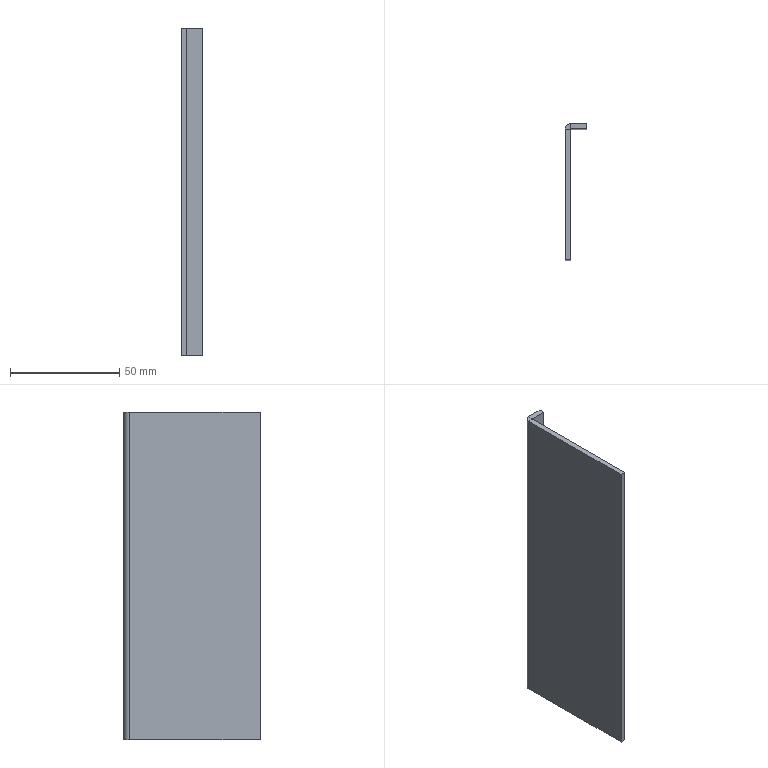Part | SolidWorks | features FlatPattern 1, SMBaseFlange 1, SheetMetal 1 | 1 solid | 14 faces | box 10 x 62.5 x 150 mm | volume 26033 mm3 | plane 12 | cylinder 2 | commonest cylinder face diameters 0.2 x1 5.2 x1
STEP:
#1=CARTESIAN_POINT('',(-7.4,0.,150.));
#2=VERTEX_POINT('',#1);
#3=CARTESIAN_POINT('',(-7.4,-2.5,150.));
#4=VERTEX_POINT('',#3);
#5=CARTESIAN_POINT('',(-7.4,0.,150.));
#6=DIRECTION('',(0.,-1.,0.));
#7=VECTOR('',#6,1000.);
#8=LINE('',#5,#7);
#9=EDGE_CURVE('',#2,#4,#8,.T.);
#10=ORIENTED_EDGE('',*,*,#9,.F.);
#11=CARTESIAN_POINT('',(-10.,-2.6,150.));
#12=VERTEX_POINT('',#11);
#13=CARTESIAN_POINT('',(-7.4,-2.6,150.));
#14=DIRECTION('',(0.,0.,1.));
#15=DIRECTION('',(-1.,0.,0.));
#16=AXIS2_PLACEMENT_3D('',#13,#14,#15);
#17=CIRCLE('',#16,2.6);
#18=EDGE_CURVE('',#2,#12,#17,.T.);
#19=ORIENTED_EDGE('',*,*,#18,.T.);
#20=CARTESIAN_POINT('',(-7.5,-2.6,150.));
#21=VERTEX_POINT('',#20);
#22=CARTESIAN_POINT('',(-7.5,-2.6,150.));
#23=DIRECTION('',(-1.,0.,0.));
#24=VECTOR('',#23,1000.);
#25=LINE('',#22,#24);
#26=EDGE_CURVE('',#21,#12,#25,.T.);
#27=ORIENTED_EDGE('',*,*,#26,.F.);
#28=CARTESIAN_POINT('',(-7.4,-2.6,150.));
#29=DIRECTION('',(0.,0.,1.));
#30=DIRECTION('',(1.,0.,0.));
#31=AXIS2_PLACEMENT_3D('',#28,#29,#30);
#32=CIRCLE('',#31,0.1);
#33=EDGE_CURVE('',#4,#21,#32,.T.);
#34=ORIENTED_EDGE('',*,*,#33,.F.);
#35=EDGE_LOOP('',(#10,#19,#27,#34));
#36=FACE_OUTER_BOUND('',#35,.T.);
#37=CARTESIAN_POINT('',(-7.4,0.,150.));
#38=DIRECTION('',(0.,0.,1.));
#39=DIRECTION('',(1.,0.,0.));
#40=AXIS2_PLACEMENT_3D('',#37,#38,#39);
#41=PLANE('',#40);
#42=ADVANCED_FACE('',(#36),#41,.T.);
#43=CARTESIAN_POINT('',(0.,0.,150.));
#44=VERTEX_POINT('',#43);
#45=CARTESIAN_POINT('',(0.,0.,150.));
#46=DIRECTION('',(-1.,0.,0.));
#47=VECTOR('',#46,1000.);
#48=LINE('',#45,#47);
#49=EDGE_CURVE('',#44,#2,#48,.T.);
#50=ORIENTED_EDGE('',*,*,#49,.T.);
#51=ORIENTED_EDGE('',*,*,#9,.T.);
#52=CARTESIAN_POINT('',(0.,-2.5,150.));
#53=VERTEX_POINT('',#52);
#54=CARTESIAN_POINT('',(0.,-2.5,150.));
#55=DIRECTION('',(-1.,0.,0.));
#56=VECTOR('',#55,1000.);
#57=LINE('',#54,#56);
#58=EDGE_CURVE('',#53,#4,#57,.T.);
#59=ORIENTED_EDGE('',*,*,#58,.F.);
#60=CARTESIAN_POINT('',(0.,0.,150.));
#61=DIRECTION('',(0.,-1.,0.));
#62=VECTOR('',#61,1000.);
#63=LINE('',#60,#62);
#64=EDGE_CURVE('',#44,#53,#63,.T.);
#65=ORIENTED_EDGE('',*,*,#64,.F.);
#66=EDGE_LOOP('',(#50,#51,#59,#65));
#67=FACE_OUTER_BOUND('',#66,.T.);
#68=CARTESIAN_POINT('',(-7.5,-2.6,150.));
#69=DIRECTION('',(0.,0.,1.));
#70=DIRECTION('',(1.,0.,0.));
#71=AXIS2_PLACEMENT_3D('',#68,#69,#70);
#72=PLANE('',#71);
#73=ADVANCED_FACE('',(#67),#72,.T.);
#74=CARTESIAN_POINT('',(-10.,-2.6,0.));
#75=VERTEX_POINT('',#74);
#76=CARTESIAN_POINT('',(-7.5,-2.6,0.));
#77=VERTEX_POINT('',#76);
#78=CARTESIAN_POINT('',(-10.,-2.6,0.));
#79=DIRECTION('',(1.,0.,0.));
#80=VECTOR('',#79,1000.);
#81=LINE('',#78,#80);
#82=EDGE_CURVE('',#75,#77,#81,.T.);
#83=ORIENTED_EDGE('',*,*,#82,.F.);
#84=CARTESIAN_POINT('',(-7.4,0.,0.));
#85=VERTEX_POINT('',#84);
#86=CARTESIAN_POINT('',(-7.4,-2.6,0.));
#87=DIRECTION('',(0.,0.,1.));
#88=DIRECTION('',(-1.,0.,0.));
#89=AXIS2_PLACEMENT_3D('',#86,#87,#88);
#90=CIRCLE('',#89,2.6);
#91=EDGE_CURVE('',#85,#75,#90,.T.);
#92=ORIENTED_EDGE('',*,*,#91,.F.);
#93=CARTESIAN_POINT('',(-7.4,-2.5,0.));
#94=VERTEX_POINT('',#93);
#95=CARTESIAN_POINT('',(-7.4,-2.5,0.));
#96=DIRECTION('',(0.,1.,0.));
#97=VECTOR('',#96,1000.);
#98=LINE('',#95,#97);
#99=EDGE_CURVE('',#94,#85,#98,.T.);
#100=ORIENTED_EDGE('',*,*,#99,.F.);
#101=CARTESIAN_POINT('',(-7.4,-2.6,0.));
#102=DIRECTION('',(0.,0.,1.));
#103=DIRECTION('',(1.,0.,0.));
#104=AXIS2_PLACEMENT_3D('',#101,#102,#103);
#105=CIRCLE('',#104,0.1);
#106=EDGE_CURVE('',#94,#77,#105,.T.);
#107=ORIENTED_EDGE('',*,*,#106,.T.);
#108=EDGE_LOOP('',(#83,#92,#100,#107));
#109=FACE_OUTER_BOUND('',#108,.T.);
#110=CARTESIAN_POINT('',(-10.,-2.6,0.));
#111=DIRECTION('',(0.,0.,-1.));
#112=DIRECTION('',(-1.,0.,0.));
#113=AXIS2_PLACEMENT_3D('',#110,#111,#112);
#114=PLANE('',#113);
#115=ADVANCED_FACE('',(#109),#114,.T.);
#116=CARTESIAN_POINT('',(-10.,-62.5,0.));
#117=VERTEX_POINT('',#116);
#118=CARTESIAN_POINT('',(-10.,0.,0.));
#119=DIRECTION('',(0.,-1.,0.));
#120=VECTOR('',#119,1000.);
#121=LINE('',#118,#120);
#122=EDGE_CURVE('',#75,#117,#121,.T.);
#123=ORIENTED_EDGE('',*,*,#122,.F.);
#124=ORIENTED_EDGE('',*,*,#82,.T.);
#125=CARTESIAN_POINT('',(-7.5,-62.5,0.));
#126=VERTEX_POINT('',#125);
#127=CARTESIAN_POINT('',(-7.5,0.,0.));
#128=DIRECTION('',(0.,-1.,0.));
#129=VECTOR('',#128,1000.);
#130=LINE('',#127,#129);
#131=EDGE_CURVE('',#77,#126,#130,.T.);
#132=ORIENTED_EDGE('',*,*,#131,.T.);
#133=CARTESIAN_POINT('',(-7.5,-62.5,0.));
#134=DIRECTION('',(-1.,0.,0.));
#135=VECTOR('',#134,1000.);
#136=LINE('',#133,#135);
#137=EDGE_CURVE('',#126,#117,#136,.T.);
#138=ORIENTED_EDGE('',*,*,#137,.T.);
#139=EDGE_LOOP('',(#123,#124,#132,#138));
#140=FACE_OUTER_BOUND('',#139,.T.);
#141=CARTESIAN_POINT('',(-7.4,-2.5,0.));
#142=DIRECTION('',(0.,0.,-1.));
#143=DIRECTION('',(-1.,0.,0.));
#144=AXIS2_PLACEMENT_3D('',#141,#142,#143);
#145=PLANE('',#144);
#146=ADVANCED_FACE('',(#140),#145,.T.);
#147=ORIENTED_EDGE('',*,*,#122,.T.);
#148=CARTESIAN_POINT('',(-10.,-62.5,150.));
#149=VERTEX_POINT('',#148);
#150=CARTESIAN_POINT('',(-10.,-62.5,150.));
#151=DIRECTION('',(0.,0.,-1.));
#152=VECTOR('',#151,1000.);
#153=LINE('',#150,#152);
#154=EDGE_CURVE('',#149,#117,#153,.T.);
#155=ORIENTED_EDGE('',*,*,#154,.F.);
#156=CARTESIAN_POINT('',(-10.,0.,150.));
#157=DIRECTION('',(0.,-1.,0.));
#158=VECTOR('',#157,1000.);
#159=LINE('',#156,#158);
#160=EDGE_CURVE('',#12,#149,#159,.T.);
#161=ORIENTED_EDGE('',*,*,#160,.F.);
#162=CARTESIAN_POINT('',(-10.,-2.6,150.));
#163=DIRECTION('',(0.,0.,-1.));
#164=VECTOR('',#163,1000.);
#165=LINE('',#162,#164);
#166=EDGE_CURVE('',#12,#75,#165,.T.);
#167=ORIENTED_EDGE('',*,*,#166,.T.);
#168=EDGE_LOOP('',(#147,#155,#161,#167));
#169=FACE_OUTER_BOUND('',#168,.T.);
#170=CARTESIAN_POINT('',(-10.,0.,150.));
#171=DIRECTION('',(1.,0.,0.));
#172=DIRECTION('',(0.,1.,0.));
#173=AXIS2_PLACEMENT_3D('',#170,#171,#172);
#174=PLANE('',#173);
#175=ADVANCED_FACE('',(#169),#174,.F.);
#176=ORIENTED_EDGE('',*,*,#137,.F.);
#177=CARTESIAN_POINT('',(-7.5,-62.5,150.));
#178=VERTEX_POINT('',#177);
#179=CARTESIAN_POINT('',(-7.5,-62.5,150.));
#180=DIRECTION('',(0.,0.,-1.));
#181=VECTOR('',#180,1000.);
#182=LINE('',#179,#181);
#183=EDGE_CURVE('',#178,#126,#182,.T.);
#184=ORIENTED_EDGE('',*,*,#183,.F.);
#185=CARTESIAN_POINT('',(-7.5,-62.5,150.));
#186=DIRECTION('',(-1.,0.,0.));
#187=VECTOR('',#186,1000.);
#188=LINE('',#185,#187);
#189=EDGE_CURVE('',#178,#149,#188,.T.);
#190=ORIENTED_EDGE('',*,*,#189,.T.);
#191=ORIENTED_EDGE('',*,*,#154,.T.);
#192=EDGE_LOOP('',(#176,#184,#190,#191));
#193=FACE_OUTER_BOUND('',#192,.T.);
#194=CARTESIAN_POINT('',(-7.5,-62.5,150.));
#195=DIRECTION('',(0.,-1.,0.));
#196=DIRECTION('',(0.,0.,-1.));
#197=AXIS2_PLACEMENT_3D('',#194,#195,#196);
#198=PLANE('',#197);
#199=ADVANCED_FACE('',(#193),#198,.T.);
#200=ORIENTED_EDGE('',*,*,#131,.F.);
#201=CARTESIAN_POINT('',(-7.5,-2.6,150.));
#202=DIRECTION('',(0.,0.,-1.));
#203=VECTOR('',#202,1000.);
#204=LINE('',#201,#203);
#205=EDGE_CURVE('',#21,#77,#204,.T.);
#206=ORIENTED_EDGE('',*,*,#205,.F.);
#207=CARTESIAN_POINT('',(-7.5,0.,150.));
#208=DIRECTION('',(0.,-1.,0.));
#209=VECTOR('',#208,1000.);
#210=LINE('',#207,#209);
#211=EDGE_CURVE('',#21,#178,#210,.T.);
#212=ORIENTED_EDGE('',*,*,#211,.T.);
#213=ORIENTED_EDGE('',*,*,#183,.T.);
#214=EDGE_LOOP('',(#200,#206,#212,#213));
#215=FACE_OUTER_BOUND('',#214,.T.);
#216=CARTESIAN_POINT('',(-7.5,0.,150.));
#217=DIRECTION('',(1.,0.,0.));
#218=DIRECTION('',(0.,1.,0.));
#219=AXIS2_PLACEMENT_3D('',#216,#217,#218);
#220=PLANE('',#219);
#221=ADVANCED_FACE('',(#215),#220,.T.);
#222=ORIENTED_EDGE('',*,*,#106,.F.);
#223=CARTESIAN_POINT('',(-7.4,-2.5,150.));
#224=DIRECTION('',(0.,0.,-1.));
#225=VECTOR('',#224,1000.);
#226=LINE('',#223,#225);
#227=EDGE_CURVE('',#4,#94,#226,.T.);
#228=ORIENTED_EDGE('',*,*,#227,.F.);
#229=ORIENTED_EDGE('',*,*,#33,.T.);
#230=ORIENTED_EDGE('',*,*,#205,.T.);
#231=EDGE_LOOP('',(#222,#228,#229,#230));
#232=FACE_OUTER_BOUND('',#231,.T.);
#233=CARTESIAN_POINT('',(-7.4,-2.6,150.));
#234=DIRECTION('',(0.,0.,-1.));
#235=DIRECTION('',(-1.,0.,0.));
#236=AXIS2_PLACEMENT_3D('',#233,#234,#235);
#237=CYLINDRICAL_SURFACE('',#236,0.1);
#238=ADVANCED_FACE('',(#232),#237,.F.);
#239=CARTESIAN_POINT('',(0.,-2.5,0.));
#240=VERTEX_POINT('',#239);
#241=CARTESIAN_POINT('',(0.,-2.5,0.));
#242=DIRECTION('',(-1.,0.,0.));
#243=VECTOR('',#242,1000.);
#244=LINE('',#241,#243);
#245=EDGE_CURVE('',#240,#94,#244,.T.);
#246=ORIENTED_EDGE('',*,*,#245,.F.);
#247=CARTESIAN_POINT('',(0.,-2.5,150.));
#248=DIRECTION('',(0.,0.,-1.));
#249=VECTOR('',#248,1000.);
#250=LINE('',#247,#249);
#251=EDGE_CURVE('',#53,#240,#250,.T.);
#252=ORIENTED_EDGE('',*,*,#251,.F.);
#253=ORIENTED_EDGE('',*,*,#58,.T.);
#254=ORIENTED_EDGE('',*,*,#227,.T.);
#255=EDGE_LOOP('',(#246,#252,#253,#254));
#256=FACE_OUTER_BOUND('',#255,.T.);
#257=CARTESIAN_POINT('',(0.,-2.5,150.));
#258=DIRECTION('',(0.,-1.,0.));
#259=DIRECTION('',(1.,0.,0.));
#260=AXIS2_PLACEMENT_3D('',#257,#258,#259);
#261=PLANE('',#260);
#262=ADVANCED_FACE('',(#256),#261,.T.);
#263=CARTESIAN_POINT('',(0.,0.,0.));
#264=VERTEX_POINT('',#263);
#265=CARTESIAN_POINT('',(0.,0.,0.));
#266=DIRECTION('',(0.,-1.,0.));
#267=VECTOR('',#266,1000.);
#268=LINE('',#265,#267);
#269=EDGE_CURVE('',#264,#240,#268,.T.);
#270=ORIENTED_EDGE('',*,*,#269,.F.);
#271=CARTESIAN_POINT('',(0.,0.,150.));
#272=DIRECTION('',(0.,0.,-1.));
#273=VECTOR('',#272,1000.);
#274=LINE('',#271,#273);
#275=EDGE_CURVE('',#44,#264,#274,.T.);
#276=ORIENTED_EDGE('',*,*,#275,.F.);
#277=ORIENTED_EDGE('',*,*,#64,.T.);
#278=ORIENTED_EDGE('',*,*,#251,.T.);
#279=EDGE_LOOP('',(#270,#276,#277,#278));
#280=FACE_OUTER_BOUND('',#279,.T.);
#281=CARTESIAN_POINT('',(0.,0.,150.));
#282=DIRECTION('',(1.,0.,0.));
#283=DIRECTION('',(0.,1.,0.));
#284=AXIS2_PLACEMENT_3D('',#281,#282,#283);
#285=PLANE('',#284);
#286=ADVANCED_FACE('',(#280),#285,.T.);
#287=CARTESIAN_POINT('',(0.,0.,0.));
#288=DIRECTION('',(-1.,0.,0.));
#289=VECTOR('',#288,1000.);
#290=LINE('',#287,#289);
#291=EDGE_CURVE('',#264,#85,#290,.T.);
#292=ORIENTED_EDGE('',*,*,#291,.T.);
#293=CARTESIAN_POINT('',(-7.4,0.,150.));
#294=DIRECTION('',(0.,0.,-1.));
#295=VECTOR('',#294,1000.);
#296=LINE('',#293,#295);
#297=EDGE_CURVE('',#2,#85,#296,.T.);
#298=ORIENTED_EDGE('',*,*,#297,.F.);
#299=ORIENTED_EDGE('',*,*,#49,.F.);
#300=ORIENTED_EDGE('',*,*,#275,.T.);
#301=EDGE_LOOP('',(#292,#298,#299,#300));
#302=FACE_OUTER_BOUND('',#301,.T.);
#303=CARTESIAN_POINT('',(0.,0.,150.));
#304=DIRECTION('',(0.,-1.,0.));
#305=DIRECTION('',(1.,0.,0.));
#306=AXIS2_PLACEMENT_3D('',#303,#304,#305);
#307=PLANE('',#306);
#308=ADVANCED_FACE('',(#302),#307,.F.);
#309=ORIENTED_EDGE('',*,*,#91,.T.);
#310=ORIENTED_EDGE('',*,*,#166,.F.);
#311=ORIENTED_EDGE('',*,*,#18,.F.);
#312=ORIENTED_EDGE('',*,*,#297,.T.);
#313=EDGE_LOOP('',(#309,#310,#311,#312));
#314=FACE_OUTER_BOUND('',#313,.T.);
#315=CARTESIAN_POINT('',(-7.4,-2.6,150.));
#316=DIRECTION('',(0.,0.,-1.));
#317=DIRECTION('',(-1.,0.,0.));
#318=AXIS2_PLACEMENT_3D('',#315,#316,#317);
#319=CYLINDRICAL_SURFACE('',#318,2.6);
#320=ADVANCED_FACE('',(#314),#319,.T.);
#321=ORIENTED_EDGE('',*,*,#160,.T.);
#322=ORIENTED_EDGE('',*,*,#189,.F.);
#323=ORIENTED_EDGE('',*,*,#211,.F.);
#324=ORIENTED_EDGE('',*,*,#26,.T.);
#325=EDGE_LOOP('',(#321,#322,#323,#324));
#326=FACE_OUTER_BOUND('',#325,.T.);
#327=CARTESIAN_POINT('',(-7.4,-2.6,150.));
#328=DIRECTION('',(0.,0.,1.));
#329=DIRECTION('',(1.,0.,0.));
#330=AXIS2_PLACEMENT_3D('',#327,#328,#329);
#331=PLANE('',#330);
#332=ADVANCED_FACE('',(#326),#331,.T.);
#333=ORIENTED_EDGE('',*,*,#245,.T.);
#334=ORIENTED_EDGE('',*,*,#99,.T.);
#335=ORIENTED_EDGE('',*,*,#291,.F.);
#336=ORIENTED_EDGE('',*,*,#269,.T.);
#337=EDGE_LOOP('',(#333,#334,#335,#336));
#338=FACE_OUTER_BOUND('',#337,.T.);
#339=CARTESIAN_POINT('',(-7.4,-2.6,0.));
#340=DIRECTION('',(0.,0.,1.));
#341=DIRECTION('',(1.,0.,0.));
#342=AXIS2_PLACEMENT_3D('',#339,#340,#341);
#343=PLANE('',#342);
#344=ADVANCED_FACE('',(#338),#343,.F.);
#345=CLOSED_SHELL('',(#42,#73,#115,#146,#175,#199,#221,#238,#262,#286,#308,#320,#332,#344));
#346=MANIFOLD_SOLID_BREP('',#345);
#347=CARTESIAN_POINT('',(0.,0.,0.));
#348=DIRECTION('',(0.,0.,1.));
#349=DIRECTION('',(1.,0.,0.));
#350=AXIS2_PLACEMENT_3D('',#347,#348,#349);
#351=(LENGTH_UNIT()NAMED_UNIT(*)SI_UNIT(.MILLI.,.METRE.));
#352=UNCERTAINTY_MEASURE_WITH_UNIT(LENGTH_MEASURE(0.00001),#351,'','');
#353=(NAMED_UNIT(*)PLANE_ANGLE_UNIT()SI_UNIT($,.RADIAN.));
#354=(NAMED_UNIT(*)SI_UNIT($,.STERADIAN.)SOLID_ANGLE_UNIT());
#355=(GEOMETRIC_REPRESENTATION_CONTEXT(3)GLOBAL_UNCERTAINTY_ASSIGNED_CONTEXT((#352))GLOBAL_UNIT_ASSIGNED_CONTEXT((#351,#353,#354))REPRESENTATION_CONTEXT('',''));
#356=ADVANCED_BREP_SHAPE_REPRESENTATION('',(#346,#350),#355);